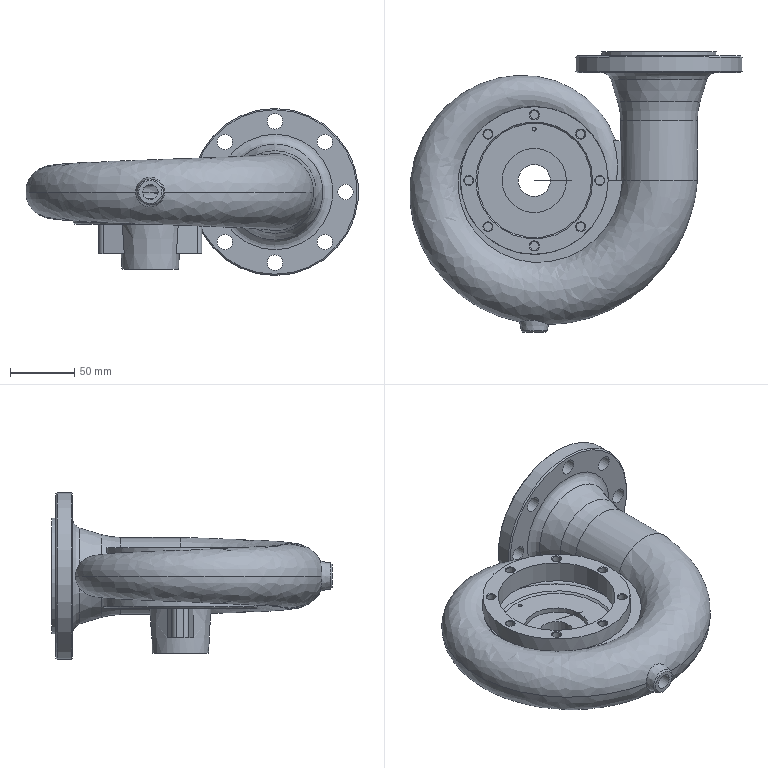Part | NX | features DATUM_CSYS 27, SKETCH 26, SIMPLE HOLE 22, SYMBOLIC_THREAD 18, EXTRUDE 17, REPLACE_FACE 15, UNITE 10, HOLE PACKAGE 9, TRIM BODY 7, CHAMFER 6, ASSOCIATIVE_INTERSECTION 5, BLEND 3, OFFSET_REGION 3, CPROJ 2, Container 2, DRAFT 2, EXTRACT_BODY 2, Geometry Instance 2, SWP104 2, DATUM_PLANE 1, SHELL 1, SKIN 1, SPLINE_LAW 1 | 1 solid | 131 faces | box 258.983 x 218 x 130 mm | volume 729840 mm3 | cylinder 44 | plane 41 | cone 39 | spline 4 | torus 3 | commonest cylinder face diameters 6.8 x16 12 x8 8 x4 3.3 x2 50 x2 3 x1